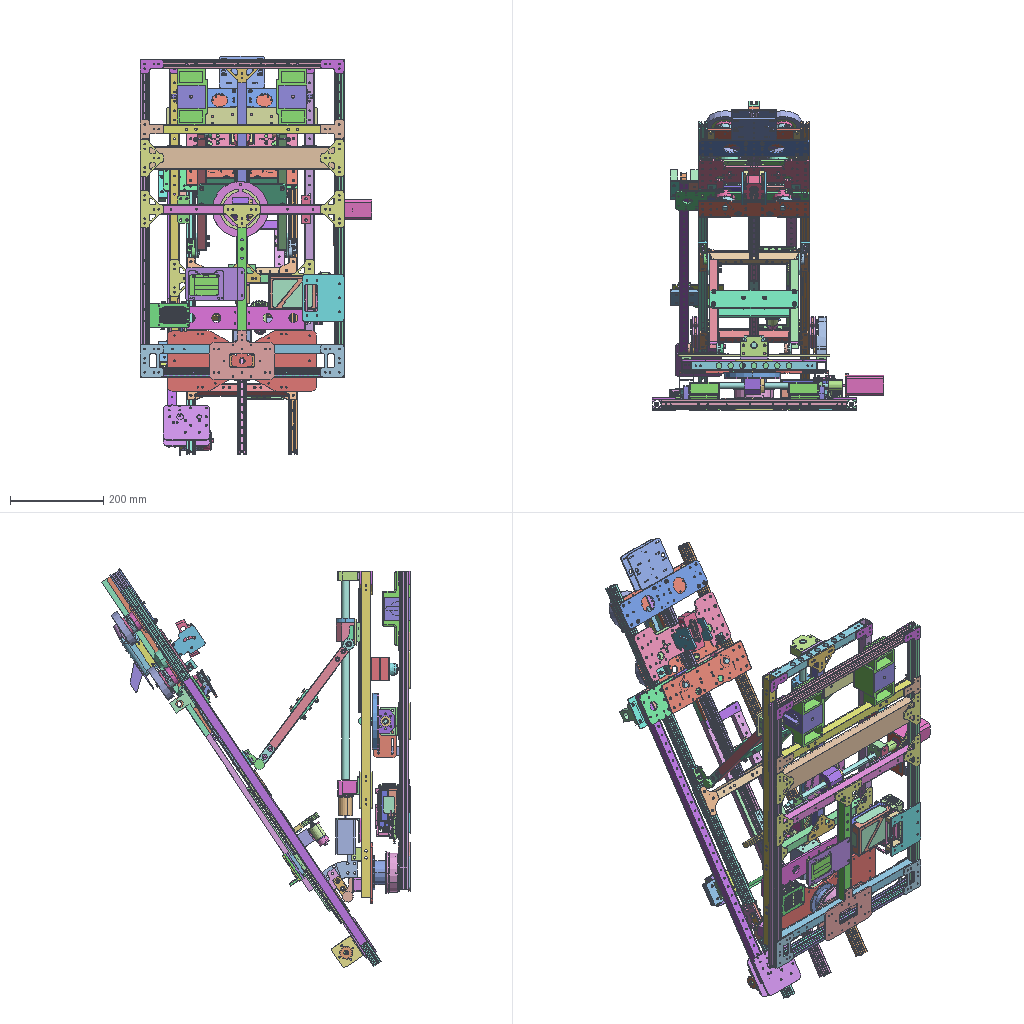Assembly | SolidWorks | 175 different items | 448 placed | box 498 x 662 x 857 mm
Parts list (item | name | quantity | parent item | size | volume | features):
1 | (subassembly) | x4 | in 9, 16 | 80 x 15 x 80 mm | 53656 mm3 | -
2 | (subassembly) | x1 | in 9 | 120 x 192.5 x 77.3 mm | 102004 mm3 | -
3 | (subassembly) | x1 | in 9 | 50.9 x 52 x 99.3 mm | 89740 mm3 | -
4 | (subassembly) | x1 | in 8 | 74.4 x 161.725 x 114.085 mm | 454834 mm3 | -
5 | (subassembly) | x1 | - | 712 x 176.326 x 325 mm | 1220944 mm3 | -
6 | (subassembly) | x1 | in 8 | 300 x 60.871 x 67.503 mm | 121134 mm3 | -
7 | (subassembly) | x1 | in 8 | 140 x 110 x 57 mm | 121657 mm3 | -
8 | (subassembly) | x1 | - | - | - | -
9 | (subassembly) | x1 | - | - | 2850499 mm3 | features CompositeCurve 1
10 | (subassembly) | x1 | - | 207.8 x 40 x 345.766 mm | 168443 mm3 | -
11 | (subassembly) | x2 | in 8 | 77 x 60 x 160 mm | 350477 mm3 | -
12 | (subassembly) | x1 | in 13 | 42 x 45 x 99.3 mm | 75357 mm3 | -
13 | (subassembly) | x1 | in 3 | 50.9 x 52 x 99.3 mm | 84016 mm3 | -
14 | (subassembly) | x1 | in 9 | 66 x 9.2 x 26 mm | 13985 mm3 | -
15 | (subassembly) | x1 | in 9 | 102 x 400 x 12 mm | 159088 mm3 | -
16 | (subassembly) | x2 | in 9 | 240 x 48 x 80 mm | 254728 mm3 | -
17 | - | x4 | in 10 | 24 x 60 x 8.2 mm | 4435 mm3 | features BaseBody 1
18 | - | x4 | in 5 | 30 x 20 x 50 mm | 4750 mm3 | features BaseBody 1
19 | - | x2 | in 5 | 50 x 27 x 20.021 mm | 8663 mm3 | features BaseBody 2
20 | - | x1 | in 5 | 310 x 4 x 50 mm | 56558 mm3 | features BaseBody 1
21 | - | x1 | in 2 | 48 x 99.2 x 42.3 mm | 57189 mm3 | features BaseBody 1
22 | - | x2 | in 4 | 16 x 16 x 36 mm | 8739 mm3 | features BaseBody 1
23 | - | x1 | in 4 | 103.5 x 55.4 x 37.5 mm | 17181 mm3 | features BaseBody 1
24 | - | x1 | in 4 | 101.5 x 44.3 x 30 mm | 74676 mm3 | features BaseBody 1
25 | - | x1 | in 4 | 37 x 106 x 68 mm | 265982 mm3 | features BaseBody 1
26 | - | x1 | in 4 | 118.5 x 22.6 x 87 mm | 22903 mm3 | features BaseBody 1
27 | - | x1 | in 4 | 118.5 x 20.1 x 87 mm | 34968 mm3 | features BaseBody 1
28 | - | x2 | in 10 | 193 x 4 x 60 mm | 45526 mm3 | features BaseBody 1
29 | - | x1 | in 9 | 73 x 77 x 2 mm | 7449 mm3 | features BaseBody 1
30 | - | x1 | in 13 | 50 x 52 x 52 mm | 8658 mm3 | features BaseBody 1
31 | - | x2 | in 9 | 20 x 20 x 90 mm | 6697 mm3 | features BaseBody 1
32 | - | x1 | in 9 | 60 x 50 x 7.5 mm | 21376 mm3 | features BaseBody 1
33 | - | x2 | in 11 | 160 x 60 x 65 mm | 180425 mm3 | features BaseBody 1
34 | - | x4 | in 8 | 40 x 3 x 50 mm | 4100 mm3 | features BaseBody 1
35 | - | x1 | in 2 | 120 x 37 x 76.843 mm | 11950 mm3 | features BaseBody 1
36 | - | x1 | in 8 | 120 x 120 x 3 mm | 29167 mm3 | features BaseBody 1
37 | - | x8 | in 5, 8 | 50 x 30 x 3 mm | 3439 mm3 | features BaseBody 1
38 | - | x2 | in 5 | 28 x 39 x 1 mm | 1004 mm3 | features BaseBody 1
39 | - | x2 | in 11 | 30 x 17.92 x 17.92 mm | 1877 mm3 | features BaseBody 1
40 | - | x1 | in 5 | 20 x 20 x 440 mm | 33241 mm3 | features BaseBody 1
41 | - | x1 | in 9 | 20 x 20 x 200 mm | 14915 mm3 | features BaseBody 1
42 | - | x1 | in 2 | 31 x 2.5 x 23 mm | 1729 mm3 | features BaseBody 1
43 | - | x1 | in 8 | 100 x 3 x 50 mm | 12708 mm3 | features BaseBody 1
44 | - | x1 | in 7 | 75 x 75 x 37 mm | 33627 mm3 | features BaseBody 1
45 | - | x4 | in 5 | 80 x 50 x 3 mm | 7139 mm3 | features BaseBody 1
46 | - | x12 | in 5, 8 | 80 x 50 x 3 mm | 7234 mm3 | features BaseBody 1
47 | - | x1 | in 7 | 90 x 90 x 2 mm | 4709 mm3 | features BaseBody 1
48 | - | x1 | in 7 | 88 x 88 x 25 mm | 37444 mm3 | features BaseBody 1
49 | - | x4 | in 8 | 70 x 50 x 3 mm | 8106 mm3 | features BaseBody 1
50 | - | x1 | in 9 | 22 x 400 x 12 mm | 79490 mm3 | features BaseBody 1
51 | - | x2 | in 8 | 65 x 5 x 20 mm | 6129 mm3 | features BaseBody 1
52 | - | x1 | in 8 | 64.5 x 3 x 60 mm | 6071 mm3 | features BaseBody 1
53 | - | x1 | in 8 | 64.75 x 3 x 60 mm | 6559 mm3 | features BaseBody 1
54 | - | x1 | in 8 | 70 x 126 x 2 mm | 11869 mm3 | features BaseBody 1
55 | - | x1 | in 8 | - | - | features BaseBody 11, RefSurface 1
56 | - | x1 | in 7 | 63 x 63 x 2 mm | 2814 mm3 | features BaseBody 1
57 | - | x1 | in 8 | 20 x 20 x 30 mm | 8586 mm3 | features BaseBody 1
58 | - | x2 | in 7, 8 | 140 x 105 x 3 mm | 29523 mm3 | features BaseBody 1
59 | - | x1 | in 8 | 438 x 682 x 20 mm | 641397 mm3 | features BaseBody 10
60 | - | x1 | in 8 | 20 x 56 x 20 mm | 4261 mm3 | features BaseBody 1
61 | - | x2 | in 15 | 22 x 400 x 12 mm | 79544 mm3 | features BaseBody 1
62 | - | x1 | in 8 | 52 x 102 x 2 mm | 6835 mm3 | features BaseBody 1
63 | - | x1 | in 8 | - | 27803 mm3 | features BaseBody 37
64 | - | x1 | in 5 | 500 x 16 x 16 mm | 97769 mm3 | features BaseBody 1
65 | - | x1 | in 5 | 320 x 5 x 130 mm | 180155 mm3 | features BaseBody 1
66 | - | x1 | in 5 | 30 x 40 x 30 mm | 23750 mm3 | features BaseBody 1
67 | - | x1 | in 5 | 40 x 47 x 48 mm | 28219 mm3 | features BaseBody 1
68 | - | x1 | in 5 | 60 x 43 x 20 mm | 40698 mm3 | features BaseBody 1
69 | - | x1 | in 5 | 60 x 34 x 42 mm | 62128 mm3 | features BaseBody 1
70 | - | x2 | in 5 | 9 x 6.5 x 260 mm | 12909 mm3 | features BaseBody 1
71 | - | x1 | in 5 | 700 x 20 x 310 mm | 144003 mm3 | features BaseBody 4
72 | - | x1 | in 9 | 240 x 20 x 1010 mm | 485681 mm3 | features BaseBody 4
73 | - | x1 | in 5 | 42.3 x 42.3 x 96.5 mm | 133444 mm3 | features BaseBody 1
74 | - | x1 | in 5 | 325 x 4 x 56 mm | 71803 mm3 | features BaseBody 1
75 | - | x1 | in 5 | 52 x 40 x 40 mm | 47312 mm3 | features BaseBody 1
76 | - | x1 | in 8 | 94 x 94 x 9 mm | 27115 mm3 | features BaseBody 1
77 | - | x1 | in 8 | 120 x 120 x 9 mm | 35937 mm3 | features BaseBody 1
78 | - | x1 | in 9 | 110 x 66 x 3 mm | 17285 mm3 | features BaseBody 1
79 | - | x1 | in 9 | 103 x 55 x 30 mm | 14827 mm3 | features BaseBody 1
80 | - | x1 | in 9 | 100 x 58 x 15 mm | 6769 mm3 | features BaseBody 1
81 | - | x1 | in 9 | 143.769 x 20.5 x 10 mm | 26301 mm3 | features BaseBody 1
82 | - | x8 | in 9 | 65 x 3 x 37.218 mm | 4717 mm3 | features BaseBody 1
83 | - | x2 | in 9 | 10 x 10 x 32 mm | 2815 mm3 | features BaseBody 1
84 | - | x1 | in 9 | 289 x 4 x 70 mm | 66384 mm3 | features BaseBody 1
85 | - | x1 | in 9 | 240 x 4 x 110 mm | 73367 mm3 | features BaseBody 1
86 | - | x1 | in 6 | 300 x 12 x 12 mm | 31011 mm3 | features BaseBody 1
87 | - | x3 | in 9 | 55 x 3 x 60 mm | 9431 mm3 | features BaseBody 1
88 | - | x1 | in 9 | 240 x 3 x 60 mm | 36133 mm3 | features BaseBody 1
89 | - | x8 | in 9 | 6.351 x 4 x 5.5 mm | 76.032 mm3 | features BaseBody 1
90 | - | x17 | in 9 | 9.238 x 5 x 8 mm | 186.691 mm3 | features BaseBody 1
91 | - | x8 | in 9 | 5.5 x 15 x 5.5 mm | 145.965 mm3 | features BaseBody 1
92 | - | x8 | in 9 | 7 x 16 x 7 mm | 289.146 mm3 | features BaseBody 1
93 | - | x18 | in 9 | 7 x 19 x 7 mm | 326.845 mm3 | features BaseBody 1
94 | - | x6 | in 9 | 8.5 x 37 x 8.5 mm | 884.331 mm3 | features BaseBody 1
95 | - | x4 | in 9 | 8.5 x 40 x 8.5 mm | 943.236 mm3 | features BaseBody 1
96 | - | x6 | in 9 | 8.5 x 45 x 8.5 mm | 1041 mm3 | features BaseBody 1
97 | - | x1 | in 6 | 50 x 35 x 36 mm | 40507 mm3 | features BaseBody 1
98 | - | x4 | in 1 | 80 x 80 x 15 mm | 35767 mm3 | features BaseBody 1
99 | - | x1 | in 9 | 51 x 24 x 18 mm | 4464 mm3 | features BaseBody 1
100 | - | x1 | in 9 | 51 x 24 x 18 mm | 4459 mm3 | features BaseBody 1
101 | - | x2 | in 9 | 24 x 60 x 8.2 mm | 4435 mm3 | features BaseBody 1
102 | - | x4 | in 9 | 54 x 3 x 48 mm | 6679 mm3 | features BaseBody 1
103 | - | x2 | in 9 | 54 x 5.5 x 48 mm | 12246 mm3 | features BaseBody 1
104 | - | x2 | in 9 | 35 x 20 x 5 mm | 3241 mm3 | features BaseBody 1
105 | - | x4 | in 1 | 58 x 15 x 58 mm | 17889 mm3 | features BaseBody 1
106 | - | x1 | in 9 | 150 x 4 x 43 mm | 19674 mm3 | features BaseBody 1
107 | - | x4 | in 9 | 35 x 3 x 60 mm | 5920 mm3 | features BaseBody 1
108 | - | x1 | in 2 | 37.988 x 192.5 x 35.318 mm | 21359 mm3 | features BaseBody 1
109 | - | x1 | in 9 | 75 x 3 x 70 mm | 15236 mm3 | features BaseBody 1
110 | - | x16 | in 9 | 7 x 10 x 7 mm | 252.82 mm3 | features BaseBody 1
111 | - | x16 | in 9 | 12 x 6 x 12 mm | 599.369 mm3 | features BaseBody 1
112 | - | x4 | in 9 | 10 x 20 x 10 mm | 1319 mm3 | features BaseBody 1
113 | - | x4 | in 9 | 70.497 x 37.1 x 70.497 mm | 35098 mm3 | features BaseBody 1
114 | - | x2 | in 9 | 20 x 32 x 20 mm | 1210 mm3 | features BaseBody 1
115 | - | x2 | in 9 | 20 x 20 x 20 mm | 753.296 mm3 | features BaseBody 1
116 | - | x2 | in 9 | 98 x 3 x 82 mm | 22758 mm3 | features BaseBody 1
117 | - | x1 | in 9 | 22.271 x 18.317 x 51.362 mm | 5366 mm3 | features BaseBody 14
118 | - | x1 | in 9 | 45 x 20 x 80 mm | 51215 mm3 | features BaseBody 1
119 | - | x3 | in 9 | 9 x 6.5 x 150 mm | 7500 mm3 | features BaseBody 1
120 | - | x2 | in 9 | 50 x 4 x 62 mm | 10165 mm3 | features BaseBody 1
121 | - | x10 | in 9 | 10 x 1 x 10 mm | 58.905 mm3 | features BaseBody 1
122 | - | x2 | in 9 | 100 x 3 x 90 mm | 25268 mm3 | features BaseBody 1
123 | - | x6 | in 9, 16 | 240 x 3 x 66 mm | 43460 mm3 | features BaseBody 1
124 | - | x1 | in 9 | 87 x 4 x 66 mm | 20382 mm3 | features BaseBody 1
125 | - | x1 | in 9 | 87 x 4 x 66 mm | 20378 mm3 | features BaseBody 1
126 | - | x1 | in 9 | 87 x 4 x 66 mm | 19855 mm3 | features BaseBody 1
127 | - | x1 | in 9 | 87 x 4 x 66 mm | 19867 mm3 | features BaseBody 1
128 | - | x4 | in 10 | 7.22 x 16 x 7.22 mm | 297.845 mm3 | features BaseBody 1
129 | - | x4 | in 10 | 8.72 x 40 x 8.72 mm | 950.488 mm3 | features BaseBody 1
130 | - | x1 | in 9 | 28 x 30 x 28 mm | 2785 mm3 | features BaseBody 1
131 | - | x12 | in 10 | 9.176 x 8 x 5 mm | 166.809 mm3 | features BaseBody 1
132 | - | x2 | in 5 | 51 x 24 x 18 mm | 4459 mm3 | features BaseBody 1
133 | - | x2 | in 5 | 51 x 24 x 18 mm | 4464 mm3 | features BaseBody 1
134 | - | x2 | in 5 | 30 x 16 x 20 mm | 8848 mm3 | features BaseBody 1
135 | - | x8 | in 10 | 30 x 10 x 10 mm | 635.279 mm3 | features BaseBody 1
136 | - | x8 | in 10 | 10 x 1 x 10 mm | 58.905 mm3 | features BaseBody 1
137 | - | x1 | in 5 | 87.153 x 20 x 95.93 mm | 65895 mm3 | features BaseBody 1
138 | - | x2 | in 2 | 64 x 2 x 14 mm | 1762 mm3 | features BaseBody 1
139 | - | x1 | in 12 | 42 x 42 x 64.3 mm | 52956 mm3 | features BaseBody 2
140 | - | x7 | in 9, 12, 16 | 42 x 45 x 43.5 mm | 22402 mm3 | features BaseBody 2
141 | - | x1 | in 9 | 64.493 x 27.178 x 34.913 mm | 21139 mm3 | features BaseBody 3
142 | - | x2 | in 11 | 72 x 55 x 50 mm | 168174 mm3 | features BaseBody 1
143 | - | x1 | in 2 | 33 x 8 x 18 mm | 4752 mm3 | features BaseBody 1
144 | - | x1 | in 6 | 60 x 39 x 20 mm | 33430 mm3 | features BaseBody 1
145 | - | x7 | in 5, 9 | 39.9 x 8 x 20 mm | 4655 mm3 | features BaseBody 1
146 | - | x1 | in 14 | 66 x 6 x 26 mm | 8148 mm3 | features BaseBody 1
147 | - | x2 | in 9 | 48 x 16 x 44 mm | 16947 mm3 | features BaseBody 1
148 | - | x1 | in 14 | 66 x 4.5 x 26 mm | 5837 mm3 | features BaseBody 1
149 | - | x1 | in 5 | 60 x 6 x 40 mm | 14094 mm3 | features BaseBody 1
150 | - | x1 | in 5 | 60 x 6 x 20 mm | 6894 mm3 | features BaseBody 1
151 | - | x2 | in 8 | 29.5 x 16 x 29.5 mm | 1637 mm3 | features BaseBody 1
152 | - | x2 | in 10 | 10 x 20 x 10 mm | 1319 mm3 | features BaseBody 1
153 | - | x1 | in 9 | 9 x 6.5 x 550 mm | 27276 mm3 | features BaseBody 1
154 | - | x1 | in 7 | 76 x 8 x 76 mm | 13540 mm3 | features BaseBody 1
155 | - | x1 | in 9 | 100 x 320 x 3 mm | 43656 mm3 | features BaseBody 1
156 | - | x1 | in 9 | 60 x 2 x 70 mm | 8139 mm3 | features BaseBody 1
157 | - | x1 | in 9 | 43.654 x 43.654 x 16 mm | 12176 mm3 | features BaseBody 1
158 | - | x2 | in 3, 9 | 28 x 28 x 14 mm | 5724 mm3 | features BaseBody 1
159 | - | x1 | in 2 | 19.6 x 11.85 x 5.5 mm | 348.463 mm3 | features BaseBody 1
160 | - | x4 | in 16 | 42 x 42 x 10 mm | 7846 mm3 | features BaseBody 1
161 | - | x1 | in 9 | 20 x 20 x 683 mm | 51247 mm3 | features BaseBody 1
162 | - | x1 | in 4 | 100 x 90 x 3 mm | 21646 mm3 | features BaseBody 1
163 | - | x1 | in 10 | 193 x 20 x 296 mm | 44469 mm3 | features BaseBody 2
164 | - | x2 | in 9 | 20 x 20 x 16 mm | 1040 mm3 | features BaseBody 1
165 | - | x14 | in 2 | 3.98 x 3.98 x 12 mm | 54.19 mm3 | features BaseBody 1
166 | - | x1 | in 5 | 53 x 51 x 50 mm | 12938 mm3 | features BaseBody 1
167 | - | x1 | in 8 | 42.3 x 42.3 x 105 mm | 139111 mm3 | features BaseBody 1
168 | - | x4 | in 2 | 10 x 3.8 x 3.8 mm | 38.4 mm3 | features BaseBody 1
169 | - | x3 | in 2 | 6 x 8.5 x 6 mm | 80.181 mm3 | features BaseBody 1
170 | - | x1 | in 9 | 22 x 10 x 400 mm | 86586 mm3 | features BaseBody 1
171 | - | x1 | in 8 | 120 x 1.5 x 120 mm | 12606 mm3 | features BaseBody 1
172 | - | x1 | in 9 | 100 x 20 x 3 mm | 5958 mm3 | features BaseBody 1
173 | - | x2 | in 5 | 9 x 6.5 x 125 mm | 6242 mm3 | features BaseBody 1
174 | - | x1 | in 6 | 30 x 42 x 42 mm | 16187 mm3 | features BaseBody 1
175 | LEB61_10-2020-10-19o | x1 | - | - | - | -
Mates (type | each side: item.copy, entity, surface, feature):
Concentric | 94.1 face cylinder Input 1 | 123.1 edge
Coincident | 107.1 face plane Input 1 | 123.1 face plane Input 1
Parallel | 107.1 face plane Input 1 | 123.1 face plane Input 1
Coincident | 123.1 face plane Input 1 | 123.2 face plane Input 1 | 2 times
Coincident | 50.1 face plane Input 1 | 21.1 face plane Input 1 | 2 times